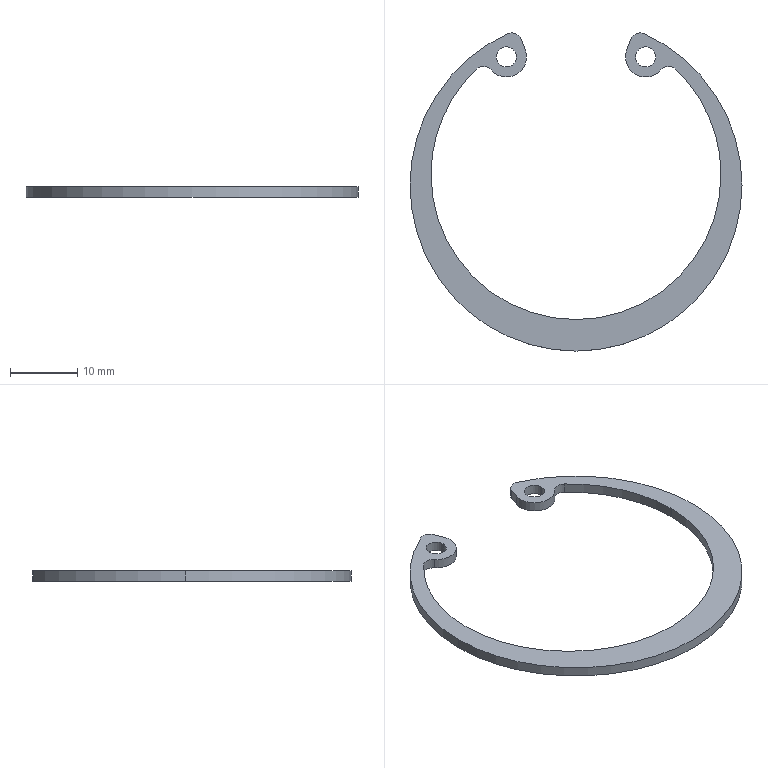Part | SolidWorks | features BaseBody 1 | 1 solid | 21 faces | box 49.5 x 47.444 x 1.5 mm | volume 686.151 mm3 | cylinder 17 | plane 4 | commonest cylinder face diameters 3 x8 6 x3 43.233 x3 49.5 x3
STEP:
#1=CARTESIAN_POINT('',(-8.881,19.113,1.5));
#2=VERTEX_POINT('',#1);
#3=CARTESIAN_POINT('',(-11.881,19.113,1.5));
#4=VERTEX_POINT('',#3);
#5=CARTESIAN_POINT('',(-10.381,19.113,1.5));
#6=DIRECTION('',(0.,0.,-1.));
#7=DIRECTION('',(-1.,0.,0.));
#8=AXIS2_PLACEMENT_3D('',#5,#6,#7);
#9=CIRCLE('',#8,1.5);
#10=EDGE_CURVE('',#2,#4,#9,.T.);
#11=ORIENTED_EDGE('',*,*,#10,.F.);
#12=CARTESIAN_POINT('',(-8.881,19.113,0.));
#13=VERTEX_POINT('',#12);
#14=CARTESIAN_POINT('',(-8.881,19.113,1.5));
#15=DIRECTION('',(0.,0.,-1.));
#16=VECTOR('',#15,1000.);
#17=LINE('',#14,#16);
#18=EDGE_CURVE('',#2,#13,#17,.T.);
#19=ORIENTED_EDGE('',*,*,#18,.T.);
#20=CARTESIAN_POINT('',(-11.881,19.113,0.));
#21=VERTEX_POINT('',#20);
#22=CARTESIAN_POINT('',(-10.381,19.113,0.));
#23=DIRECTION('',(0.,0.,1.));
#24=DIRECTION('',(-1.,0.,0.));
#25=AXIS2_PLACEMENT_3D('',#22,#23,#24);
#26=CIRCLE('',#25,1.5);
#27=EDGE_CURVE('',#21,#13,#26,.T.);
#28=ORIENTED_EDGE('',*,*,#27,.F.);
#29=CARTESIAN_POINT('',(-11.881,19.113,1.5));
#30=DIRECTION('',(0.,0.,-1.));
#31=VECTOR('',#30,1000.);
#32=LINE('',#29,#31);
#33=EDGE_CURVE('',#4,#21,#32,.T.);
#34=ORIENTED_EDGE('',*,*,#33,.F.);
#35=EDGE_LOOP('',(#11,#19,#28,#34));
#36=FACE_OUTER_BOUND('',#35,.T.);
#37=CARTESIAN_POINT('',(-10.381,19.113,1.5));
#38=DIRECTION('',(0.,0.,-1.));
#39=DIRECTION('',(-1.,0.,0.));
#40=AXIS2_PLACEMENT_3D('',#37,#38,#39);
#41=CYLINDRICAL_SURFACE('',#40,1.5);
#42=ADVANCED_FACE('',(#36),#41,.F.);
#43=CARTESIAN_POINT('',(11.881,19.113,1.5));
#44=VERTEX_POINT('',#43);
#45=CARTESIAN_POINT('',(8.881,19.113,1.5));
#46=VERTEX_POINT('',#45);
#47=CARTESIAN_POINT('',(10.381,19.113,1.5));
#48=DIRECTION('',(0.,0.,-1.));
#49=DIRECTION('',(-1.,0.,0.));
#50=AXIS2_PLACEMENT_3D('',#47,#48,#49);
#51=CIRCLE('',#50,1.5);
#52=EDGE_CURVE('',#44,#46,#51,.T.);
#53=ORIENTED_EDGE('',*,*,#52,.F.);
#54=CARTESIAN_POINT('',(11.881,19.113,0.));
#55=VERTEX_POINT('',#54);
#56=CARTESIAN_POINT('',(11.881,19.113,1.5));
#57=DIRECTION('',(0.,0.,-1.));
#58=VECTOR('',#57,1000.);
#59=LINE('',#56,#58);
#60=EDGE_CURVE('',#44,#55,#59,.T.);
#61=ORIENTED_EDGE('',*,*,#60,.T.);
#62=CARTESIAN_POINT('',(8.881,19.113,0.));
#63=VERTEX_POINT('',#62);
#64=CARTESIAN_POINT('',(10.381,19.113,0.));
#65=DIRECTION('',(0.,0.,1.));
#66=DIRECTION('',(-1.,0.,0.));
#67=AXIS2_PLACEMENT_3D('',#64,#65,#66);
#68=CIRCLE('',#67,1.5);
#69=EDGE_CURVE('',#63,#55,#68,.T.);
#70=ORIENTED_EDGE('',*,*,#69,.F.);
#71=CARTESIAN_POINT('',(8.881,19.113,1.5));
#72=DIRECTION('',(0.,0.,-1.));
#73=VECTOR('',#72,1000.);
#74=LINE('',#71,#73);
#75=EDGE_CURVE('',#46,#63,#74,.T.);
#76=ORIENTED_EDGE('',*,*,#75,.F.);
#77=EDGE_LOOP('',(#53,#61,#70,#76));
#78=FACE_OUTER_BOUND('',#77,.T.);
#79=CARTESIAN_POINT('',(10.381,19.113,1.5));
#80=DIRECTION('',(0.,0.,-1.));
#81=DIRECTION('',(-1.,0.,0.));
#82=AXIS2_PLACEMENT_3D('',#79,#80,#81);
#83=CYLINDRICAL_SURFACE('',#82,1.5);
#84=ADVANCED_FACE('',(#78),#83,.F.);
#85=CARTESIAN_POINT('',(-12.666,17.168,0.));
#86=VERTEX_POINT('',#85);
#87=CARTESIAN_POINT('',(-7.381,19.113,0.));
#88=VERTEX_POINT('',#87);
#89=CARTESIAN_POINT('',(-10.381,19.113,0.));
#90=DIRECTION('',(0.,0.,1.));
#91=DIRECTION('',(1.,0.,0.));
#92=AXIS2_PLACEMENT_3D('',#89,#90,#91);
#93=CIRCLE('',#92,3.);
#94=EDGE_CURVE('',#86,#88,#93,.T.);
#95=ORIENTED_EDGE('',*,*,#94,.T.);
#96=CARTESIAN_POINT('',(-7.381,19.113,1.5));
#97=VERTEX_POINT('',#96);
#98=CARTESIAN_POINT('',(-7.381,19.113,1.5));
#99=DIRECTION('',(0.,0.,1.));
#100=VECTOR('',#99,1000.);
#101=LINE('',#98,#100);
#102=EDGE_CURVE('',#88,#97,#101,.T.);
#103=ORIENTED_EDGE('',*,*,#102,.T.);
#104=CARTESIAN_POINT('',(-12.666,17.168,1.5));
#105=VERTEX_POINT('',#104);
#106=CARTESIAN_POINT('',(-10.381,19.113,1.5));
#107=DIRECTION('',(0.,0.,1.));
#108=DIRECTION('',(1.,0.,0.));
#109=AXIS2_PLACEMENT_3D('',#106,#107,#108);
#110=CIRCLE('',#109,3.);
#111=EDGE_CURVE('',#105,#97,#110,.T.);
#112=ORIENTED_EDGE('',*,*,#111,.F.);
#113=CARTESIAN_POINT('',(-12.666,17.168,1.5));
#114=DIRECTION('',(0.,0.,-1.));
#115=VECTOR('',#114,1000.);
#116=LINE('',#113,#115);
#117=EDGE_CURVE('',#105,#86,#116,.T.);
#118=ORIENTED_EDGE('',*,*,#117,.T.);
#119=EDGE_LOOP('',(#95,#103,#112,#118));
#120=FACE_OUTER_BOUND('',#119,.T.);
#121=CARTESIAN_POINT('',(-10.381,19.113,1.5));
#122=DIRECTION('',(0.,0.,1.));
#123=DIRECTION('',(1.,0.,0.));
#124=AXIS2_PLACEMENT_3D('',#121,#122,#123);
#125=CYLINDRICAL_SURFACE('',#124,3.);
#126=ADVANCED_FACE('',(#120),#125,.T.);
#127=CARTESIAN_POINT('',(-21.617,1.567,0.));
#128=VERTEX_POINT('',#127);
#129=CARTESIAN_POINT('',(21.617,1.567,0.));
#130=VERTEX_POINT('',#129);
#131=CARTESIAN_POINT('',(0.,1.567,0.));
#132=DIRECTION('',(0.,0.,1.));
#133=DIRECTION('',(1.,0.,0.));
#134=AXIS2_PLACEMENT_3D('',#131,#132,#133);
#135=CIRCLE('',#134,21.617);
#136=EDGE_CURVE('',#128,#130,#135,.T.);
#137=ORIENTED_EDGE('',*,*,#136,.F.);
#138=CARTESIAN_POINT('',(-21.617,1.567,1.5));
#139=VERTEX_POINT('',#138);
#140=CARTESIAN_POINT('',(-21.617,1.567,1.5));
#141=DIRECTION('',(0.,0.,1.));
#142=VECTOR('',#141,1000.);
#143=LINE('',#140,#142);
#144=EDGE_CURVE('',#128,#139,#143,.T.);
#145=ORIENTED_EDGE('',*,*,#144,.T.);
#146=CARTESIAN_POINT('',(21.617,1.567,1.5));
#147=VERTEX_POINT('',#146);
#148=CARTESIAN_POINT('',(0.,1.567,1.5));
#149=DIRECTION('',(0.,0.,-1.));
#150=DIRECTION('',(1.,0.,0.));
#151=AXIS2_PLACEMENT_3D('',#148,#149,#150);
#152=CIRCLE('',#151,21.617);
#153=EDGE_CURVE('',#147,#139,#152,.T.);
#154=ORIENTED_EDGE('',*,*,#153,.F.);
#155=CARTESIAN_POINT('',(21.617,1.567,1.5));
#156=DIRECTION('',(0.,0.,1.));
#157=VECTOR('',#156,1000.);
#158=LINE('',#155,#157);
#159=EDGE_CURVE('',#130,#147,#158,.T.);
#160=ORIENTED_EDGE('',*,*,#159,.F.);
#161=EDGE_LOOP('',(#137,#145,#154,#160));
#162=FACE_OUTER_BOUND('',#161,.T.);
#163=CARTESIAN_POINT('',(0.,1.567,1.5));
#164=DIRECTION('',(0.,0.,1.));
#165=DIRECTION('',(1.,0.,0.));
#166=AXIS2_PLACEMENT_3D('',#163,#164,#165);
#167=CYLINDRICAL_SURFACE('',#166,21.617);
#168=ADVANCED_FACE('',(#162),#167,.F.);
#169=CARTESIAN_POINT('',(14.837,17.287,0.));
#170=VERTEX_POINT('',#169);
#171=CARTESIAN_POINT('',(0.,1.567,0.));
#172=DIRECTION('',(0.,0.,1.));
#173=DIRECTION('',(1.,0.,0.));
#174=AXIS2_PLACEMENT_3D('',#171,#172,#173);
#175=CIRCLE('',#174,21.617);
#176=EDGE_CURVE('',#130,#170,#175,.T.);
#177=ORIENTED_EDGE('',*,*,#176,.F.);
#178=ORIENTED_EDGE('',*,*,#159,.T.);
#179=CARTESIAN_POINT('',(14.837,17.287,1.5));
#180=VERTEX_POINT('',#179);
#181=CARTESIAN_POINT('',(0.,1.567,1.5));
#182=DIRECTION('',(0.,0.,-1.));
#183=DIRECTION('',(1.,0.,0.));
#184=AXIS2_PLACEMENT_3D('',#181,#182,#183);
#185=CIRCLE('',#184,21.617);
#186=EDGE_CURVE('',#180,#147,#185,.T.);
#187=ORIENTED_EDGE('',*,*,#186,.F.);
#188=CARTESIAN_POINT('',(14.837,17.287,1.5));
#189=DIRECTION('',(0.,0.,1.));
#190=VECTOR('',#189,1000.);
#191=LINE('',#188,#190);
#192=EDGE_CURVE('',#170,#180,#191,.T.);
#193=ORIENTED_EDGE('',*,*,#192,.F.);
#194=EDGE_LOOP('',(#177,#178,#187,#193));
#195=FACE_OUTER_BOUND('',#194,.T.);
#196=CARTESIAN_POINT('',(0.,1.567,1.5));
#197=DIRECTION('',(0.,0.,1.));
#198=DIRECTION('',(1.,0.,0.));
#199=AXIS2_PLACEMENT_3D('',#196,#197,#198);
#200=CYLINDRICAL_SURFACE('',#199,21.617);
#201=ADVANCED_FACE('',(#195),#200,.F.);
#202=CARTESIAN_POINT('',(-10.177,22.561,0.));
#203=VERTEX_POINT('',#202);
#204=CARTESIAN_POINT('',(-24.75,0.,0.));
#205=VERTEX_POINT('',#204);
#206=CARTESIAN_POINT('',(0.,0.,0.));
#207=DIRECTION('',(0.,0.,1.));
#208=DIRECTION('',(1.,0.,0.));
#209=AXIS2_PLACEMENT_3D('',#206,#207,#208);
#210=CIRCLE('',#209,24.75);
#211=EDGE_CURVE('',#203,#205,#210,.T.);
#212=ORIENTED_EDGE('',*,*,#211,.T.);
#213=CARTESIAN_POINT('',(-24.75,0.,1.5));
#214=VERTEX_POINT('',#213);
#215=CARTESIAN_POINT('',(-24.75,0.,0.));
#216=DIRECTION('',(0.,0.,1.));
#217=VECTOR('',#216,1000.);
#218=LINE('',#215,#217);
#219=EDGE_CURVE('',#205,#214,#218,.T.);
#220=ORIENTED_EDGE('',*,*,#219,.T.);
#221=CARTESIAN_POINT('',(-10.177,22.561,1.5));
#222=VERTEX_POINT('',#221);
#223=CARTESIAN_POINT('',(0.,0.,1.5));
#224=DIRECTION('',(0.,0.,1.));
#225=DIRECTION('',(1.,0.,0.));
#226=AXIS2_PLACEMENT_3D('',#223,#224,#225);
#227=CIRCLE('',#226,24.75);
#228=EDGE_CURVE('',#222,#214,#227,.T.);
#229=ORIENTED_EDGE('',*,*,#228,.F.);
#230=CARTESIAN_POINT('',(-10.177,22.561,0.));
#231=DIRECTION('',(0.,0.,-1.));
#232=VECTOR('',#231,1000.);
#233=LINE('',#230,#232);
#234=EDGE_CURVE('',#222,#203,#233,.T.);
#235=ORIENTED_EDGE('',*,*,#234,.T.);
#236=EDGE_LOOP('',(#212,#220,#229,#235));
#237=FACE_OUTER_BOUND('',#236,.T.);
#238=CARTESIAN_POINT('',(0.,0.,0.));
#239=DIRECTION('',(0.,0.,1.));
#240=DIRECTION('',(1.,0.,0.));
#241=AXIS2_PLACEMENT_3D('',#238,#239,#240);
#242=CYLINDRICAL_SURFACE('',#241,24.75);
#243=ADVANCED_FACE('',(#237),#242,.T.);
#244=ORIENTED_EDGE('',*,*,#219,.F.);
#245=CARTESIAN_POINT('',(24.75,0.,0.));
#246=VERTEX_POINT('',#245);
#247=CARTESIAN_POINT('',(0.,0.,0.));
#248=DIRECTION('',(0.,0.,1.));
#249=DIRECTION('',(1.,0.,0.));
#250=AXIS2_PLACEMENT_3D('',#247,#248,#249);
#251=CIRCLE('',#250,24.75);
#252=EDGE_CURVE('',#205,#246,#251,.T.);
#253=ORIENTED_EDGE('',*,*,#252,.T.);
#254=CARTESIAN_POINT('',(24.75,0.,1.5));
#255=VERTEX_POINT('',#254);
#256=CARTESIAN_POINT('',(24.75,0.,0.));
#257=DIRECTION('',(0.,0.,1.));
#258=VECTOR('',#257,1000.);
#259=LINE('',#256,#258);
#260=EDGE_CURVE('',#246,#255,#259,.T.);
#261=ORIENTED_EDGE('',*,*,#260,.T.);
#262=CARTESIAN_POINT('',(0.,0.,1.5));
#263=DIRECTION('',(0.,0.,1.));
#264=DIRECTION('',(1.,0.,0.));
#265=AXIS2_PLACEMENT_3D('',#262,#263,#264);
#266=CIRCLE('',#265,24.75);
#267=EDGE_CURVE('',#214,#255,#266,.T.);
#268=ORIENTED_EDGE('',*,*,#267,.F.);
#269=EDGE_LOOP('',(#244,#253,#261,#268));
#270=FACE_OUTER_BOUND('',#269,.T.);
#271=CARTESIAN_POINT('',(0.,0.,0.));
#272=DIRECTION('',(0.,0.,1.));
#273=DIRECTION('',(1.,0.,0.));
#274=AXIS2_PLACEMENT_3D('',#271,#272,#273);
#275=CYLINDRICAL_SURFACE('',#274,24.75);
#276=ADVANCED_FACE('',(#270),#275,.T.);
#277=CARTESIAN_POINT('',(-10.381,19.113,1.5));
#278=DIRECTION('',(0.,0.,-1.));
#279=DIRECTION('',(-1.,0.,0.));
#280=AXIS2_PLACEMENT_3D('',#277,#278,#279);
#281=CIRCLE('',#280,1.5);
#282=EDGE_CURVE('',#4,#2,#281,.T.);
#283=ORIENTED_EDGE('',*,*,#282,.T.);
#284=ORIENTED_EDGE('',*,*,#10,.T.);
#285=EDGE_LOOP('',(#283,#284));
#286=FACE_BOUND('',#285,.T.);
#287=CARTESIAN_POINT('',(10.381,19.113,1.5));
#288=DIRECTION('',(0.,0.,-1.));
#289=DIRECTION('',(-1.,0.,0.));
#290=AXIS2_PLACEMENT_3D('',#287,#288,#289);
#291=CIRCLE('',#290,1.5);
#292=EDGE_CURVE('',#46,#44,#291,.T.);
#293=ORIENTED_EDGE('',*,*,#292,.T.);
#294=ORIENTED_EDGE('',*,*,#52,.T.);
#295=EDGE_LOOP('',(#293,#294));
#296=FACE_BOUND('',#295,.T.);
#297=ORIENTED_EDGE('',*,*,#111,.T.);
#298=CARTESIAN_POINT('',(-7.572,20.167,1.5));
#299=VERTEX_POINT('',#298);
#300=CARTESIAN_POINT('',(-10.381,19.113,1.5));
#301=DIRECTION('',(0.,0.,1.));
#302=DIRECTION('',(1.,0.,0.));
#303=AXIS2_PLACEMENT_3D('',#300,#301,#302);
#304=CIRCLE('',#303,3.);
#305=EDGE_CURVE('',#97,#299,#304,.T.);
#306=ORIENTED_EDGE('',*,*,#305,.T.);
#307=CARTESIAN_POINT('',(-8.156,21.721,1.5));
#308=VERTEX_POINT('',#307);
#309=CARTESIAN_POINT('',(-7.572,20.167,1.5));
#310=DIRECTION('',(-0.3515,0.9362,0.));
#311=VECTOR('',#310,1000.);
#312=LINE('',#309,#311);
#313=EDGE_CURVE('',#299,#308,#312,.T.);
#314=ORIENTED_EDGE('',*,*,#313,.T.);
#315=CARTESIAN_POINT('',(-9.56,21.194,1.5));
#316=DIRECTION('',(0.,0.,1.));
#317=DIRECTION('',(1.,0.,0.));
#318=AXIS2_PLACEMENT_3D('',#315,#316,#317);
#319=CIRCLE('',#318,1.5);
#320=EDGE_CURVE('',#308,#222,#319,.T.);
#321=ORIENTED_EDGE('',*,*,#320,.T.);
#322=ORIENTED_EDGE('',*,*,#228,.T.);
#323=ORIENTED_EDGE('',*,*,#267,.T.);
#324=CARTESIAN_POINT('',(10.177,22.561,1.5));
#325=VERTEX_POINT('',#324);
#326=CARTESIAN_POINT('',(0.,0.,1.5));
#327=DIRECTION('',(0.,0.,1.));
#328=DIRECTION('',(1.,0.,0.));
#329=AXIS2_PLACEMENT_3D('',#326,#327,#328);
#330=CIRCLE('',#329,24.75);
#331=EDGE_CURVE('',#255,#325,#330,.T.);
#332=ORIENTED_EDGE('',*,*,#331,.T.);
#333=CARTESIAN_POINT('',(8.156,21.721,1.5));
#334=VERTEX_POINT('',#333);
#335=CARTESIAN_POINT('',(9.56,21.194,1.5));
#336=DIRECTION('',(0.,0.,1.));
#337=DIRECTION('',(-1.,0.,0.));
#338=AXIS2_PLACEMENT_3D('',#335,#336,#337);
#339=CIRCLE('',#338,1.5);
#340=EDGE_CURVE('',#325,#334,#339,.T.);
#341=ORIENTED_EDGE('',*,*,#340,.T.);
#342=CARTESIAN_POINT('',(7.572,20.167,1.5));
#343=VERTEX_POINT('',#342);
#344=CARTESIAN_POINT('',(8.156,21.721,1.5));
#345=DIRECTION('',(-0.3515,-0.9362,0.));
#346=VECTOR('',#345,1000.);
#347=LINE('',#344,#346);
#348=EDGE_CURVE('',#334,#343,#347,.T.);
#349=ORIENTED_EDGE('',*,*,#348,.T.);
#350=CARTESIAN_POINT('',(12.666,17.168,1.5));
#351=VERTEX_POINT('',#350);
#352=CARTESIAN_POINT('',(10.381,19.113,1.5));
#353=DIRECTION('',(0.,0.,1.));
#354=DIRECTION('',(1.,0.,0.));
#355=AXIS2_PLACEMENT_3D('',#352,#353,#354);
#356=CIRCLE('',#355,3.);
#357=EDGE_CURVE('',#343,#351,#356,.T.);
#358=ORIENTED_EDGE('',*,*,#357,.T.);
#359=CARTESIAN_POINT('',(13.808,16.196,1.5));
#360=DIRECTION('',(0.,0.,-1.));
#361=DIRECTION('',(-1.,0.,0.));
#362=AXIS2_PLACEMENT_3D('',#359,#360,#361);
#363=CIRCLE('',#362,1.5);
#364=EDGE_CURVE('',#351,#180,#363,.T.);
#365=ORIENTED_EDGE('',*,*,#364,.T.);
#366=ORIENTED_EDGE('',*,*,#186,.T.);
#367=ORIENTED_EDGE('',*,*,#153,.T.);
#368=CARTESIAN_POINT('',(-14.837,17.287,1.5));
#369=VERTEX_POINT('',#368);
#370=CARTESIAN_POINT('',(0.,1.567,1.5));
#371=DIRECTION('',(0.,0.,-1.));
#372=DIRECTION('',(1.,0.,0.));
#373=AXIS2_PLACEMENT_3D('',#370,#371,#372);
#374=CIRCLE('',#373,21.617);
#375=EDGE_CURVE('',#139,#369,#374,.T.);
#376=ORIENTED_EDGE('',*,*,#375,.T.);
#377=CARTESIAN_POINT('',(-13.808,16.196,1.5));
#378=DIRECTION('',(0.,0.,-1.));
#379=DIRECTION('',(-1.,0.,0.));
#380=AXIS2_PLACEMENT_3D('',#377,#378,#379);
#381=CIRCLE('',#380,1.5);
#382=EDGE_CURVE('',#369,#105,#381,.T.);
#383=ORIENTED_EDGE('',*,*,#382,.T.);
#384=EDGE_LOOP('',(#297,#306,#314,#321,#322,#323,#332,#341,#349,#358,#365,#366,#367,#376,#383));
#385=FACE_OUTER_BOUND('',#384,.T.);
#386=CARTESIAN_POINT('',(0.,0.,1.5));
#387=DIRECTION('',(0.,0.,1.));
#388=DIRECTION('',(1.,0.,0.));
#389=AXIS2_PLACEMENT_3D('',#386,#387,#388);
#390=PLANE('',#389);
#391=ADVANCED_FACE('',(#286,#296,#385),#390,.T.);
#392=ORIENTED_EDGE('',*,*,#18,.F.);
#393=ORIENTED_EDGE('',*,*,#282,.F.);
#394=ORIENTED_EDGE('',*,*,#33,.T.);
#395=CARTESIAN_POINT('',(-10.381,19.113,0.));
#396=DIRECTION('',(0.,0.,1.));
#397=DIRECTION('',(-1.,0.,0.));
#398=AXIS2_PLACEMENT_3D('',#395,#396,#397);
#399=CIRCLE('',#398,1.5);
#400=EDGE_CURVE('',#13,#21,#399,.T.);
#401=ORIENTED_EDGE('',*,*,#400,.F.);
#402=EDGE_LOOP('',(#392,#393,#394,#401));
#403=FACE_OUTER_BOUND('',#402,.T.);
#404=CARTESIAN_POINT('',(-10.381,19.113,1.5));
#405=DIRECTION('',(0.,0.,-1.));
#406=DIRECTION('',(-1.,0.,0.));
#407=AXIS2_PLACEMENT_3D('',#404,#405,#406);
#408=CYLINDRICAL_SURFACE('',#407,1.5);
#409=ADVANCED_FACE('',(#403),#408,.F.);
#410=ORIENTED_EDGE('',*,*,#60,.F.);
#411=ORIENTED_EDGE('',*,*,#292,.F.);
#412=ORIENTED_EDGE('',*,*,#75,.T.);
#413=CARTESIAN_POINT('',(10.381,19.113,0.));
#414=DIRECTION('',(0.,0.,1.));
#415=DIRECTION('',(-1.,0.,0.));
#416=AXIS2_PLACEMENT_3D('',#413,#414,#415);
#417=CIRCLE('',#416,1.5);
#418=EDGE_CURVE('',#55,#63,#417,.T.);
#419=ORIENTED_EDGE('',*,*,#418,.F.);
#420=EDGE_LOOP('',(#410,#411,#412,#419));
#421=FACE_OUTER_BOUND('',#420,.T.);
#422=CARTESIAN_POINT('',(10.381,19.113,1.5));
#423=DIRECTION('',(0.,0.,-1.));
#424=DIRECTION('',(-1.,0.,0.));
#425=AXIS2_PLACEMENT_3D('',#422,#423,#424);
#426=CYLINDRICAL_SURFACE('',#425,1.5);
#427=ADVANCED_FACE('',(#421),#426,.F.);
#428=ORIENTED_EDGE('',*,*,#313,.F.);
#429=CARTESIAN_POINT('',(-7.572,20.167,0.));
#430=VERTEX_POINT('',#429);
#431=CARTESIAN_POINT('',(-7.572,20.167,1.5));
#432=DIRECTION('',(0.,0.,1.));
#433=VECTOR('',#432,1000.);
#434=LINE('',#431,#433);
#435=EDGE_CURVE('',#430,#299,#434,.T.);
#436=ORIENTED_EDGE('',*,*,#435,.F.);
#437=CARTESIAN_POINT('',(-8.156,21.721,0.));
#438=VERTEX_POINT('',#437);
#439=CARTESIAN_POINT('',(-8.7,23.171,0.));
#440=DIRECTION('',(0.3515,-0.9362,0.));
#441=VECTOR('',#440,1000.);
#442=LINE('',#439,#441);
#443=EDGE_CURVE('',#438,#430,#442,.T.);
#444=ORIENTED_EDGE('',*,*,#443,.F.);
#445=CARTESIAN_POINT('',(-8.156,21.721,1.5));
#446=DIRECTION('',(0.,0.,-1.));
#447=VECTOR('',#446,1000.);
#448=LINE('',#445,#447);
#449=EDGE_CURVE('',#308,#438,#448,.T.);
#450=ORIENTED_EDGE('',*,*,#449,.F.);
#451=EDGE_LOOP('',(#428,#436,#444,#450));
#452=FACE_OUTER_BOUND('',#451,.T.);
#453=CARTESIAN_POINT('',(-8.7,23.171,1.5));
#454=DIRECTION('',(-0.9362,-0.3515,0.));
#455=DIRECTION('',(0.3515,-0.9362,0.));
#456=AXIS2_PLACEMENT_3D('',#453,#454,#455);
#457=PLANE('',#456);
#458=ADVANCED_FACE('',(#452),#457,.F.);
#459=ORIENTED_EDGE('',*,*,#102,.F.);
#460=CARTESIAN_POINT('',(-10.381,19.113,0.));
#461=DIRECTION('',(0.,0.,1.));
#462=DIRECTION('',(1.,0.,0.));
#463=AXIS2_PLACEMENT_3D('',#460,#461,#462);
#464=CIRCLE('',#463,3.);
#465=EDGE_CURVE('',#88,#430,#464,.T.);
#466=ORIENTED_EDGE('',*,*,#465,.T.);
#467=ORIENTED_EDGE('',*,*,#435,.T.);
#468=ORIENTED_EDGE('',*,*,#305,.F.);
#469=EDGE_LOOP('',(#459,#466,#467,#468));
#470=FACE_OUTER_BOUND('',#469,.T.);
#471=CARTESIAN_POINT('',(-10.381,19.113,1.5));
#472=DIRECTION('',(0.,0.,1.));
#473=DIRECTION('',(1.,0.,0.));
#474=AXIS2_PLACEMENT_3D('',#471,#472,#473);
#475=CYLINDRICAL_SURFACE('',#474,3.);
#476=ADVANCED_FACE('',(#470),#475,.T.);
#477=ORIENTED_EDGE('',*,*,#117,.F.);
#478=ORIENTED_EDGE('',*,*,#382,.F.);
#479=CARTESIAN_POINT('',(-14.837,17.287,0.));
#480=VERTEX_POINT('',#479);
#481=CARTESIAN_POINT('',(-14.837,17.287,1.5));
#482=DIRECTION('',(0.,0.,1.));
#483=VECTOR('',#482,1000.);
#484=LINE('',#481,#483);
#485=EDGE_CURVE('',#480,#369,#484,.T.);
#486=ORIENTED_EDGE('',*,*,#485,.F.);
#487=CARTESIAN_POINT('',(-13.808,16.196,0.));
#488=DIRECTION('',(0.,0.,1.));
#489=DIRECTION('',(-1.,0.,0.));
#490=AXIS2_PLACEMENT_3D('',#487,#488,#489);
#491=CIRCLE('',#490,1.5);
#492=EDGE_CURVE('',#86,#480,#491,.T.);
#493=ORIENTED_EDGE('',*,*,#492,.F.);
#494=EDGE_LOOP('',(#477,#478,#486,#493));
#495=FACE_OUTER_BOUND('',#494,.T.);
#496=CARTESIAN_POINT('',(-13.808,16.196,1.5));
#497=DIRECTION('',(0.,0.,-1.));
#498=DIRECTION('',(-1.,0.,0.));
#499=AXIS2_PLACEMENT_3D('',#496,#497,#498);
#500=CYLINDRICAL_SURFACE('',#499,1.5);
#501=ADVANCED_FACE('',(#495),#500,.F.);
#502=ORIENTED_EDGE('',*,*,#144,.F.);
#503=CARTESIAN_POINT('',(0.,1.567,0.));
#504=DIRECTION('',(0.,0.,1.));
#505=DIRECTION('',(1.,0.,0.));
#506=AXIS2_PLACEMENT_3D('',#503,#504,#505);
#507=CIRCLE('',#506,21.617);
#508=EDGE_CURVE('',#480,#128,#507,.T.);
#509=ORIENTED_EDGE('',*,*,#508,.F.);
#510=ORIENTED_EDGE('',*,*,#485,.T.);
#511=ORIENTED_EDGE('',*,*,#375,.F.);
#512=EDGE_LOOP('',(#502,#509,#510,#511));
#513=FACE_OUTER_BOUND('',#512,.T.);
#514=CARTESIAN_POINT('',(0.,1.567,1.5));
#515=DIRECTION('',(0.,0.,1.));
#516=DIRECTION('',(1.,0.,0.));
#517=AXIS2_PLACEMENT_3D('',#514,#515,#516);
#518=CYLINDRICAL_SURFACE('',#517,21.617);
#519=ADVANCED_FACE('',(#513),#518,.F.);
#520=ORIENTED_EDGE('',*,*,#192,.T.);
#521=ORIENTED_EDGE('',*,*,#364,.F.);
#522=CARTESIAN_POINT('',(12.666,17.168,0.));
#523=VERTEX_POINT('',#522);
#524=CARTESIAN_POINT('',(12.666,17.168,1.5));
#525=DIRECTION('',(0.,0.,1.));
#526=VECTOR('',#525,1000.);
#527=LINE('',#524,#526);
#528=EDGE_CURVE('',#523,#351,#527,.T.);
#529=ORIENTED_EDGE('',*,*,#528,.F.);
#530=CARTESIAN_POINT('',(13.808,16.196,0.));
#531=DIRECTION('',(0.,0.,1.));
#532=DIRECTION('',(-1.,0.,0.));
#533=AXIS2_PLACEMENT_3D('',#530,#531,#532);
#534=CIRCLE('',#533,1.5);
#535=EDGE_CURVE('',#170,#523,#534,.T.);
#536=ORIENTED_EDGE('',*,*,#535,.F.);
#537=EDGE_LOOP('',(#520,#521,#529,#536));
#538=FACE_OUTER_BOUND('',#537,.T.);
#539=CARTESIAN_POINT('',(13.808,16.196,1.5));
#540=DIRECTION('',(0.,0.,-1.));
#541=DIRECTION('',(-1.,0.,0.));
#542=AXIS2_PLACEMENT_3D('',#539,#540,#541);
#543=CYLINDRICAL_SURFACE('',#542,1.5);
#544=ADVANCED_FACE('',(#538),#543,.F.);
#545=CARTESIAN_POINT('',(7.572,20.167,0.));
#546=VERTEX_POINT('',#545);
#547=CARTESIAN_POINT('',(7.572,20.167,1.5));
#548=DIRECTION('',(0.,0.,-1.));
#549=VECTOR('',#548,1000.);
#550=LINE('',#547,#549);
#551=EDGE_CURVE('',#343,#546,#550,.T.);
#552=ORIENTED_EDGE('',*,*,#551,.T.);
#553=CARTESIAN_POINT('',(10.381,19.113,0.));
#554=DIRECTION('',(0.,0.,1.));
#555=DIRECTION('',(1.,0.,0.));
#556=AXIS2_PLACEMENT_3D('',#553,#554,#555);
#557=CIRCLE('',#556,3.);
#558=EDGE_CURVE('',#546,#523,#557,.T.);
#559=ORIENTED_EDGE('',*,*,#558,.T.);
#560=ORIENTED_EDGE('',*,*,#528,.T.);
#561=ORIENTED_EDGE('',*,*,#357,.F.);
#562=EDGE_LOOP('',(#552,#559,#560,#561));
#563=FACE_OUTER_BOUND('',#562,.T.);
#564=CARTESIAN_POINT('',(10.381,19.113,1.5));
#565=DIRECTION('',(0.,0.,1.));
#566=DIRECTION('',(1.,0.,0.));
#567=AXIS2_PLACEMENT_3D('',#564,#565,#566);
#568=CYLINDRICAL_SURFACE('',#567,3.);
#569=ADVANCED_FACE('',(#563),#568,.T.);
#570=ORIENTED_EDGE('',*,*,#348,.F.);
#571=CARTESIAN_POINT('',(8.156,21.721,0.));
#572=VERTEX_POINT('',#571);
#573=CARTESIAN_POINT('',(8.156,21.721,1.5));
#574=DIRECTION('',(0.,0.,1.));
#575=VECTOR('',#574,1000.);
#576=LINE('',#573,#575);
#577=EDGE_CURVE('',#572,#334,#576,.T.);
#578=ORIENTED_EDGE('',*,*,#577,.F.);
#579=CARTESIAN_POINT('',(7.572,20.167,0.));
#580=DIRECTION('',(0.3515,0.9362,0.));
#581=VECTOR('',#580,1000.);
#582=LINE('',#579,#581);
#583=EDGE_CURVE('',#546,#572,#582,.T.);
#584=ORIENTED_EDGE('',*,*,#583,.F.);
#585=ORIENTED_EDGE('',*,*,#551,.F.);
#586=EDGE_LOOP('',(#570,#578,#584,#585));
#587=FACE_OUTER_BOUND('',#586,.T.);
#588=CARTESIAN_POINT('',(7.572,20.167,1.5));
#589=DIRECTION('',(0.9362,-0.3515,0.));
#590=DIRECTION('',(0.3515,0.9362,0.));
#591=AXIS2_PLACEMENT_3D('',#588,#589,#590);
#592=PLANE('',#591);
#593=ADVANCED_FACE('',(#587),#592,.F.);
#594=CARTESIAN_POINT('',(10.177,22.561,0.));
#595=VERTEX_POINT('',#594);
#596=CARTESIAN_POINT('',(9.56,21.194,0.));
#597=DIRECTION('',(0.,0.,1.));
#598=DIRECTION('',(-1.,0.,0.));
#599=AXIS2_PLACEMENT_3D('',#596,#597,#598);
#600=CIRCLE('',#599,1.5);
#601=EDGE_CURVE('',#595,#572,#600,.T.);
#602=ORIENTED_EDGE('',*,*,#601,.T.);
#603=ORIENTED_EDGE('',*,*,#577,.T.);
#604=ORIENTED_EDGE('',*,*,#340,.F.);
#605=CARTESIAN_POINT('',(10.177,22.561,0.));
#606=DIRECTION('',(0.,0.,-1.));
#607=VECTOR('',#606,1000.);
#608=LINE('',#605,#607);
#609=EDGE_CURVE('',#325,#595,#608,.T.);
#610=ORIENTED_EDGE('',*,*,#609,.T.);
#611=EDGE_LOOP('',(#602,#603,#604,#610));
#612=FACE_OUTER_BOUND('',#611,.T.);
#613=CARTESIAN_POINT('',(9.56,21.194,0.));
#614=DIRECTION('',(0.,0.,-1.));
#615=DIRECTION('',(-1.,0.,0.));
#616=AXIS2_PLACEMENT_3D('',#613,#614,#615);
#617=CYLINDRICAL_SURFACE('',#616,1.5);
#618=ADVANCED_FACE('',(#612),#617,.T.);
#619=ORIENTED_EDGE('',*,*,#260,.F.);
#620=CARTESIAN_POINT('',(0.,0.,0.));
#621=DIRECTION('',(0.,0.,1.));
#622=DIRECTION('',(1.,0.,0.));
#623=AXIS2_PLACEMENT_3D('',#620,#621,#622);
#624=CIRCLE('',#623,24.75);
#625=EDGE_CURVE('',#246,#595,#624,.T.);
#626=ORIENTED_EDGE('',*,*,#625,.T.);
#627=ORIENTED_EDGE('',*,*,#609,.F.);
#628=ORIENTED_EDGE('',*,*,#331,.F.);
#629=EDGE_LOOP('',(#619,#626,#627,#628));
#630=FACE_OUTER_BOUND('',#629,.T.);
#631=CARTESIAN_POINT('',(0.,0.,0.));
#632=DIRECTION('',(0.,0.,1.));
#633=DIRECTION('',(1.,0.,0.));
#634=AXIS2_PLACEMENT_3D('',#631,#632,#633);
#635=CYLINDRICAL_SURFACE('',#634,24.75);
#636=ADVANCED_FACE('',(#630),#635,.T.);
#637=ORIENTED_EDGE('',*,*,#320,.F.);
#638=ORIENTED_EDGE('',*,*,#449,.T.);
#639=CARTESIAN_POINT('',(-9.56,21.194,0.));
#640=DIRECTION('',(0.,0.,1.));
#641=DIRECTION('',(1.,0.,0.));
#642=AXIS2_PLACEMENT_3D('',#639,#640,#641);
#643=CIRCLE('',#642,1.5);
#644=EDGE_CURVE('',#438,#203,#643,.T.);
#645=ORIENTED_EDGE('',*,*,#644,.T.);
#646=ORIENTED_EDGE('',*,*,#234,.F.);
#647=EDGE_LOOP('',(#637,#638,#645,#646));
#648=FACE_OUTER_BOUND('',#647,.T.);
#649=CARTESIAN_POINT('',(-9.56,21.194,0.));
#650=DIRECTION('',(0.,0.,1.));
#651=DIRECTION('',(1.,0.,0.));
#652=AXIS2_PLACEMENT_3D('',#649,#650,#651);
#653=CYLINDRICAL_SURFACE('',#652,1.5);
#654=ADVANCED_FACE('',(#648),#653,.T.);
#655=ORIENTED_EDGE('',*,*,#27,.T.);
#656=ORIENTED_EDGE('',*,*,#400,.T.);
#657=EDGE_LOOP('',(#655,#656));
#658=FACE_BOUND('',#657,.T.);
#659=ORIENTED_EDGE('',*,*,#69,.T.);
#660=ORIENTED_EDGE('',*,*,#418,.T.);
#661=EDGE_LOOP('',(#659,#660));
#662=FACE_BOUND('',#661,.T.);
#663=ORIENTED_EDGE('',*,*,#492,.T.);
#664=ORIENTED_EDGE('',*,*,#508,.T.);
#665=ORIENTED_EDGE('',*,*,#136,.T.);
#666=ORIENTED_EDGE('',*,*,#176,.T.);
#667=ORIENTED_EDGE('',*,*,#535,.T.);
#668=ORIENTED_EDGE('',*,*,#558,.F.);
#669=ORIENTED_EDGE('',*,*,#583,.T.);
#670=ORIENTED_EDGE('',*,*,#601,.F.);
#671=ORIENTED_EDGE('',*,*,#625,.F.);
#672=ORIENTED_EDGE('',*,*,#252,.F.);
#673=ORIENTED_EDGE('',*,*,#211,.F.);
#674=ORIENTED_EDGE('',*,*,#644,.F.);
#675=ORIENTED_EDGE('',*,*,#443,.T.);
#676=ORIENTED_EDGE('',*,*,#465,.F.);
#677=ORIENTED_EDGE('',*,*,#94,.F.);
#678=EDGE_LOOP('',(#663,#664,#665,#666,#667,#668,#669,#670,#671,#672,#673,#674,#675,#676,#677));
#679=FACE_OUTER_BOUND('',#678,.T.);
#680=CARTESIAN_POINT('',(0.,0.,0.));
#681=DIRECTION('',(0.,0.,1.));
#682=DIRECTION('',(1.,0.,0.));
#683=AXIS2_PLACEMENT_3D('',#680,#681,#682);
#684=PLANE('',#683);
#685=ADVANCED_FACE('',(#658,#662,#679),#684,.F.);
#686=CLOSED_SHELL('',(#42,#84,#126,#168,#201,#243,#276,#391,#409,#427,#458,#476,#501,#519,#544,#569,#593,#618,#636,#654,#685));
#687=MANIFOLD_SOLID_BREP('',#686);
#688=CARTESIAN_POINT('',(0.,0.,0.));
#689=DIRECTION('',(0.,0.,1.));
#690=DIRECTION('',(1.,0.,0.));
#691=AXIS2_PLACEMENT_3D('',#688,#689,#690);
#692=(LENGTH_UNIT()NAMED_UNIT(*)SI_UNIT(.MILLI.,.METRE.));
#693=UNCERTAINTY_MEASURE_WITH_UNIT(LENGTH_MEASURE(0.00001),#692,'','');
#694=(NAMED_UNIT(*)PLANE_ANGLE_UNIT()SI_UNIT($,.RADIAN.));
#695=(NAMED_UNIT(*)SI_UNIT($,.STERADIAN.)SOLID_ANGLE_UNIT());
#696=(GEOMETRIC_REPRESENTATION_CONTEXT(3)GLOBAL_UNCERTAINTY_ASSIGNED_CONTEXT((#693))GLOBAL_UNIT_ASSIGNED_CONTEXT((#692,#694,#695))REPRESENTATION_CONTEXT('',''));
#697=ADVANCED_BREP_SHAPE_REPRESENTATION('',(#687,#691),#696);